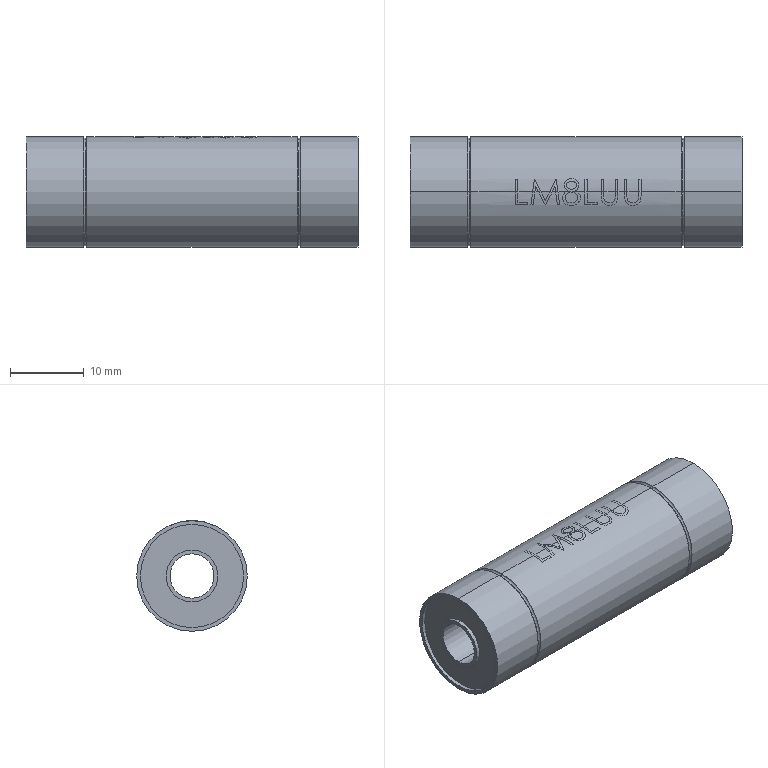Part | SolidWorks | features Emboss 1, Revolution 1 | 1 solid | 54 faces | box 45 x 15 x 15 mm | volume 6555 mm3 | cylinder 40 | torus 8 | plane 6 | commonest cylinder face diameters 15 x30 7 x4 14 x4 6 x2